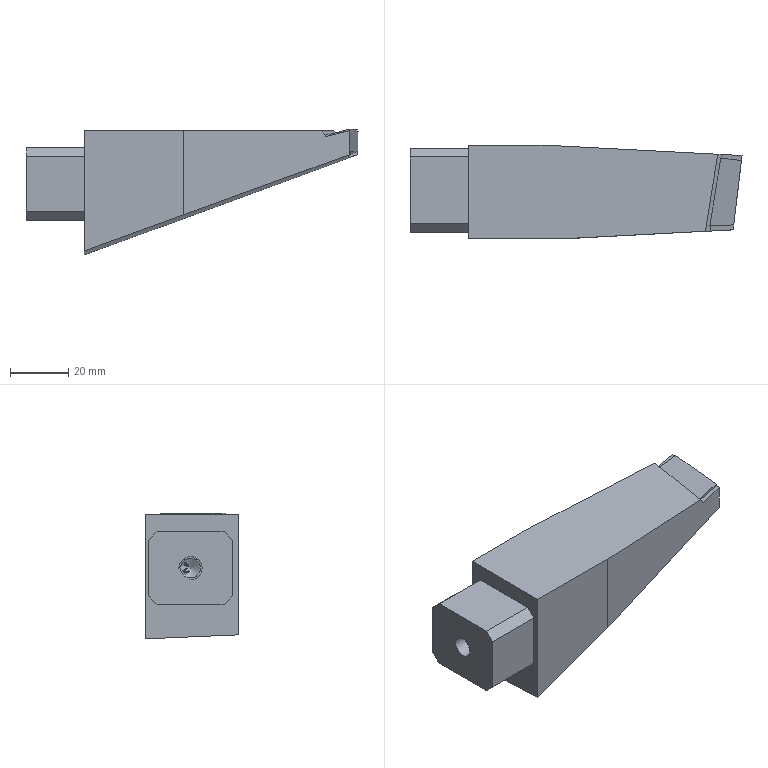Part | STEP file | P011002S003-001 | 1 solid | 62 faces | box 113.977 x 32 x 43.155 mm | volume 84322 mm3 | plane 36 | other 10 | cone 7 | spline 6 | cylinder 3 | commonest cylinder face diameters 6.8 x1 7.973 x1 8 x1